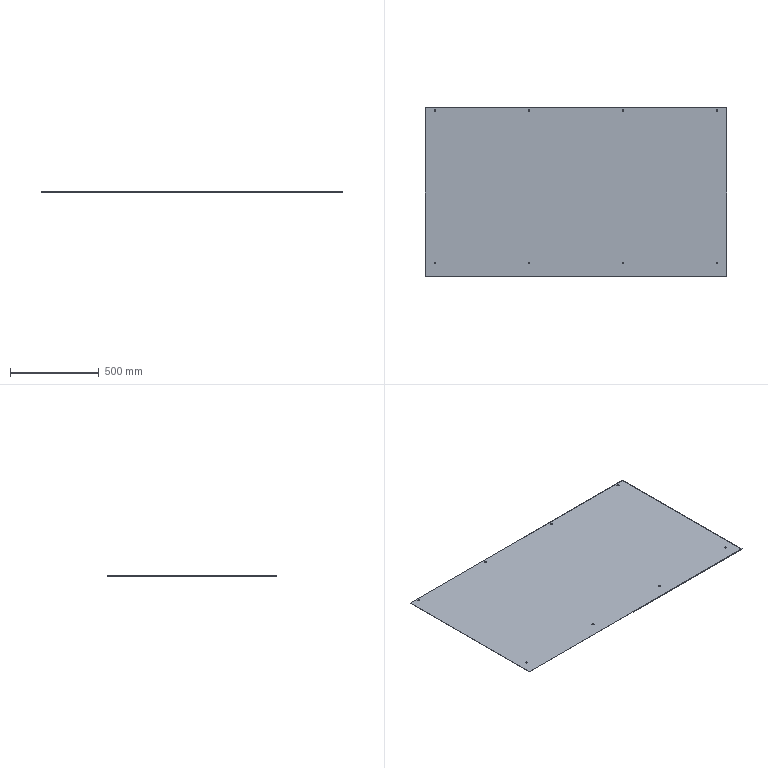Part | SolidWorks | features ICE 2, Extrusion 1 | 1 solid | 24 faces | box 1700 x 950 x 3 mm | volume 4835265 mm3 | cone 16 | plane 8
STEP:
#1=CARTESIAN_POINT('',(-261.75,460.,3.));
#2=VERTEX_POINT('',#1);
#3=CARTESIAN_POINT('',(-268.25,460.,3.));
#4=VERTEX_POINT('',#3);
#5=CARTESIAN_POINT('',(-265.,460.,3.));
#6=DIRECTION('',(0.,0.,1.));
#7=DIRECTION('',(1.,0.,0.));
#8=AXIS2_PLACEMENT_3D('',#5,#6,#7);
#9=CIRCLE('',#8,3.25);
#10=EDGE_CURVE('',#2,#4,#9,.T.);
#11=ORIENTED_EDGE('',*,*,#10,.T.);
#12=CARTESIAN_POINT('',(-271.25,460.,0.));
#13=VERTEX_POINT('',#12);
#14=CARTESIAN_POINT('',(-268.25,460.,3.));
#15=DIRECTION('',(-0.7071,0.,-0.7071));
#16=VECTOR('',#15,1000.);
#17=LINE('',#14,#16);
#18=EDGE_CURVE('',#4,#13,#17,.T.);
#19=ORIENTED_EDGE('',*,*,#18,.T.);
#20=CARTESIAN_POINT('',(-258.75,460.,0.));
#21=VERTEX_POINT('',#20);
#22=CARTESIAN_POINT('',(-265.,460.,0.));
#23=DIRECTION('',(0.,0.,1.));
#24=DIRECTION('',(1.,0.,0.));
#25=AXIS2_PLACEMENT_3D('',#22,#23,#24);
#26=CIRCLE('',#25,6.25);
#27=EDGE_CURVE('',#21,#13,#26,.T.);
#28=ORIENTED_EDGE('',*,*,#27,.F.);
#29=CARTESIAN_POINT('',(-261.75,460.,3.));
#30=DIRECTION('',(0.7071,0.,-0.7071));
#31=VECTOR('',#30,1000.);
#32=LINE('',#29,#31);
#33=EDGE_CURVE('',#2,#21,#32,.T.);
#34=ORIENTED_EDGE('',*,*,#33,.F.);
#35=EDGE_LOOP('',(#11,#19,#28,#34));
#36=FACE_OUTER_BOUND('',#35,.T.);
#37=CARTESIAN_POINT('',(-265.,460.,3.));
#38=DIRECTION('',(0.,0.,-1.));
#39=DIRECTION('',(1.,0.,0.));
#40=AXIS2_PLACEMENT_3D('',#37,#38,#39);
#41=CONICAL_SURFACE('',#40,3.25,0.7854);
#42=ADVANCED_FACE('',(#36),#41,.F.);
#43=CARTESIAN_POINT('',(268.25,460.,3.));
#44=VERTEX_POINT('',#43);
#45=CARTESIAN_POINT('',(261.75,460.,3.));
#46=VERTEX_POINT('',#45);
#47=CARTESIAN_POINT('',(265.,460.,3.));
#48=DIRECTION('',(0.,0.,1.));
#49=DIRECTION('',(1.,0.,0.));
#50=AXIS2_PLACEMENT_3D('',#47,#48,#49);
#51=CIRCLE('',#50,3.25);
#52=EDGE_CURVE('',#44,#46,#51,.T.);
#53=ORIENTED_EDGE('',*,*,#52,.T.);
#54=CARTESIAN_POINT('',(258.75,460.,0.));
#55=VERTEX_POINT('',#54);
#56=CARTESIAN_POINT('',(261.75,460.,3.));
#57=DIRECTION('',(-0.7071,0.,-0.7071));
#58=VECTOR('',#57,1000.);
#59=LINE('',#56,#58);
#60=EDGE_CURVE('',#46,#55,#59,.T.);
#61=ORIENTED_EDGE('',*,*,#60,.T.);
#62=CARTESIAN_POINT('',(271.25,460.,0.));
#63=VERTEX_POINT('',#62);
#64=CARTESIAN_POINT('',(265.,460.,0.));
#65=DIRECTION('',(0.,0.,1.));
#66=DIRECTION('',(1.,0.,0.));
#67=AXIS2_PLACEMENT_3D('',#64,#65,#66);
#68=CIRCLE('',#67,6.25);
#69=EDGE_CURVE('',#63,#55,#68,.T.);
#70=ORIENTED_EDGE('',*,*,#69,.F.);
#71=CARTESIAN_POINT('',(268.25,460.,3.));
#72=DIRECTION('',(0.7071,0.,-0.7071));
#73=VECTOR('',#72,1000.);
#74=LINE('',#71,#73);
#75=EDGE_CURVE('',#44,#63,#74,.T.);
#76=ORIENTED_EDGE('',*,*,#75,.F.);
#77=EDGE_LOOP('',(#53,#61,#70,#76));
#78=FACE_OUTER_BOUND('',#77,.T.);
#79=CARTESIAN_POINT('',(265.,460.,3.));
#80=DIRECTION('',(0.,0.,-1.));
#81=DIRECTION('',(1.,0.,0.));
#82=AXIS2_PLACEMENT_3D('',#79,#80,#81);
#83=CONICAL_SURFACE('',#82,3.25,0.7854);
#84=ADVANCED_FACE('',(#78),#83,.F.);
#85=CARTESIAN_POINT('',(798.25,460.,3.));
#86=VERTEX_POINT('',#85);
#87=CARTESIAN_POINT('',(791.75,460.,3.));
#88=VERTEX_POINT('',#87);
#89=CARTESIAN_POINT('',(795.,460.,3.));
#90=DIRECTION('',(0.,0.,1.));
#91=DIRECTION('',(1.,0.,0.));
#92=AXIS2_PLACEMENT_3D('',#89,#90,#91);
#93=CIRCLE('',#92,3.25);
#94=EDGE_CURVE('',#86,#88,#93,.T.);
#95=ORIENTED_EDGE('',*,*,#94,.T.);
#96=CARTESIAN_POINT('',(788.75,460.,0.));
#97=VERTEX_POINT('',#96);
#98=CARTESIAN_POINT('',(791.75,460.,3.));
#99=DIRECTION('',(-0.7071,0.,-0.7071));
#100=VECTOR('',#99,1000.);
#101=LINE('',#98,#100);
#102=EDGE_CURVE('',#88,#97,#101,.T.);
#103=ORIENTED_EDGE('',*,*,#102,.T.);
#104=CARTESIAN_POINT('',(801.25,460.,0.));
#105=VERTEX_POINT('',#104);
#106=CARTESIAN_POINT('',(795.,460.,0.));
#107=DIRECTION('',(0.,0.,1.));
#108=DIRECTION('',(1.,0.,0.));
#109=AXIS2_PLACEMENT_3D('',#106,#107,#108);
#110=CIRCLE('',#109,6.25);
#111=EDGE_CURVE('',#105,#97,#110,.T.);
#112=ORIENTED_EDGE('',*,*,#111,.F.);
#113=CARTESIAN_POINT('',(798.25,460.,3.));
#114=DIRECTION('',(0.7071,0.,-0.7071));
#115=VECTOR('',#114,1000.);
#116=LINE('',#113,#115);
#117=EDGE_CURVE('',#86,#105,#116,.T.);
#118=ORIENTED_EDGE('',*,*,#117,.F.);
#119=EDGE_LOOP('',(#95,#103,#112,#118));
#120=FACE_OUTER_BOUND('',#119,.T.);
#121=CARTESIAN_POINT('',(795.,460.,3.));
#122=DIRECTION('',(0.,0.,-1.));
#123=DIRECTION('',(1.,0.,0.));
#124=AXIS2_PLACEMENT_3D('',#121,#122,#123);
#125=CONICAL_SURFACE('',#124,3.25,0.7854);
#126=ADVANCED_FACE('',(#120),#125,.F.);
#127=CARTESIAN_POINT('',(798.25,-400.,3.));
#128=VERTEX_POINT('',#127);
#129=CARTESIAN_POINT('',(791.75,-400.,3.));
#130=VERTEX_POINT('',#129);
#131=CARTESIAN_POINT('',(795.,-400.,3.));
#132=DIRECTION('',(0.,0.,1.));
#133=DIRECTION('',(1.,0.,0.));
#134=AXIS2_PLACEMENT_3D('',#131,#132,#133);
#135=CIRCLE('',#134,3.25);
#136=EDGE_CURVE('',#128,#130,#135,.T.);
#137=ORIENTED_EDGE('',*,*,#136,.T.);
#138=CARTESIAN_POINT('',(788.75,-400.,0.));
#139=VERTEX_POINT('',#138);
#140=CARTESIAN_POINT('',(791.75,-400.,3.));
#141=DIRECTION('',(-0.7071,0.,-0.7071));
#142=VECTOR('',#141,1000.);
#143=LINE('',#140,#142);
#144=EDGE_CURVE('',#130,#139,#143,.T.);
#145=ORIENTED_EDGE('',*,*,#144,.T.);
#146=CARTESIAN_POINT('',(801.25,-400.,0.));
#147=VERTEX_POINT('',#146);
#148=CARTESIAN_POINT('',(795.,-400.,0.));
#149=DIRECTION('',(0.,0.,1.));
#150=DIRECTION('',(1.,0.,0.));
#151=AXIS2_PLACEMENT_3D('',#148,#149,#150);
#152=CIRCLE('',#151,6.25);
#153=EDGE_CURVE('',#147,#139,#152,.T.);
#154=ORIENTED_EDGE('',*,*,#153,.F.);
#155=CARTESIAN_POINT('',(798.25,-400.,3.));
#156=DIRECTION('',(0.7071,0.,-0.7071));
#157=VECTOR('',#156,1000.);
#158=LINE('',#155,#157);
#159=EDGE_CURVE('',#128,#147,#158,.T.);
#160=ORIENTED_EDGE('',*,*,#159,.F.);
#161=EDGE_LOOP('',(#137,#145,#154,#160));
#162=FACE_OUTER_BOUND('',#161,.T.);
#163=CARTESIAN_POINT('',(795.,-400.,3.));
#164=DIRECTION('',(0.,0.,-1.));
#165=DIRECTION('',(1.,0.,0.));
#166=AXIS2_PLACEMENT_3D('',#163,#164,#165);
#167=CONICAL_SURFACE('',#166,3.25,0.7854);
#168=ADVANCED_FACE('',(#162),#167,.F.);
#169=CARTESIAN_POINT('',(268.25,-400.,3.));
#170=VERTEX_POINT('',#169);
#171=CARTESIAN_POINT('',(261.75,-400.,3.));
#172=VERTEX_POINT('',#171);
#173=CARTESIAN_POINT('',(265.,-400.,3.));
#174=DIRECTION('',(0.,0.,1.));
#175=DIRECTION('',(1.,0.,0.));
#176=AXIS2_PLACEMENT_3D('',#173,#174,#175);
#177=CIRCLE('',#176,3.25);
#178=EDGE_CURVE('',#170,#172,#177,.T.);
#179=ORIENTED_EDGE('',*,*,#178,.T.);
#180=CARTESIAN_POINT('',(258.75,-400.,0.));
#181=VERTEX_POINT('',#180);
#182=CARTESIAN_POINT('',(261.75,-400.,3.));
#183=DIRECTION('',(-0.7071,0.,-0.7071));
#184=VECTOR('',#183,1000.);
#185=LINE('',#182,#184);
#186=EDGE_CURVE('',#172,#181,#185,.T.);
#187=ORIENTED_EDGE('',*,*,#186,.T.);
#188=CARTESIAN_POINT('',(271.25,-400.,0.));
#189=VERTEX_POINT('',#188);
#190=CARTESIAN_POINT('',(265.,-400.,0.));
#191=DIRECTION('',(0.,0.,1.));
#192=DIRECTION('',(1.,0.,0.));
#193=AXIS2_PLACEMENT_3D('',#190,#191,#192);
#194=CIRCLE('',#193,6.25);
#195=EDGE_CURVE('',#189,#181,#194,.T.);
#196=ORIENTED_EDGE('',*,*,#195,.F.);
#197=CARTESIAN_POINT('',(268.25,-400.,3.));
#198=DIRECTION('',(0.7071,0.,-0.7071));
#199=VECTOR('',#198,1000.);
#200=LINE('',#197,#199);
#201=EDGE_CURVE('',#170,#189,#200,.T.);
#202=ORIENTED_EDGE('',*,*,#201,.F.);
#203=EDGE_LOOP('',(#179,#187,#196,#202));
#204=FACE_OUTER_BOUND('',#203,.T.);
#205=CARTESIAN_POINT('',(265.,-400.,3.));
#206=DIRECTION('',(0.,0.,-1.));
#207=DIRECTION('',(1.,0.,0.));
#208=AXIS2_PLACEMENT_3D('',#205,#206,#207);
#209=CONICAL_SURFACE('',#208,3.25,0.7854);
#210=ADVANCED_FACE('',(#204),#209,.F.);
#211=CARTESIAN_POINT('',(-261.75,-400.,3.));
#212=VERTEX_POINT('',#211);
#213=CARTESIAN_POINT('',(-268.25,-400.,3.));
#214=VERTEX_POINT('',#213);
#215=CARTESIAN_POINT('',(-265.,-400.,3.));
#216=DIRECTION('',(0.,0.,1.));
#217=DIRECTION('',(1.,0.,0.));
#218=AXIS2_PLACEMENT_3D('',#215,#216,#217);
#219=CIRCLE('',#218,3.25);
#220=EDGE_CURVE('',#212,#214,#219,.T.);
#221=ORIENTED_EDGE('',*,*,#220,.T.);
#222=CARTESIAN_POINT('',(-271.25,-400.,0.));
#223=VERTEX_POINT('',#222);
#224=CARTESIAN_POINT('',(-268.25,-400.,3.));
#225=DIRECTION('',(-0.7071,0.,-0.7071));
#226=VECTOR('',#225,1000.);
#227=LINE('',#224,#226);
#228=EDGE_CURVE('',#214,#223,#227,.T.);
#229=ORIENTED_EDGE('',*,*,#228,.T.);
#230=CARTESIAN_POINT('',(-258.75,-400.,0.));
#231=VERTEX_POINT('',#230);
#232=CARTESIAN_POINT('',(-265.,-400.,0.));
#233=DIRECTION('',(0.,0.,1.));
#234=DIRECTION('',(1.,0.,0.));
#235=AXIS2_PLACEMENT_3D('',#232,#233,#234);
#236=CIRCLE('',#235,6.25);
#237=EDGE_CURVE('',#231,#223,#236,.T.);
#238=ORIENTED_EDGE('',*,*,#237,.F.);
#239=CARTESIAN_POINT('',(-261.75,-400.,3.));
#240=DIRECTION('',(0.7071,0.,-0.7071));
#241=VECTOR('',#240,1000.);
#242=LINE('',#239,#241);
#243=EDGE_CURVE('',#212,#231,#242,.T.);
#244=ORIENTED_EDGE('',*,*,#243,.F.);
#245=EDGE_LOOP('',(#221,#229,#238,#244));
#246=FACE_OUTER_BOUND('',#245,.T.);
#247=CARTESIAN_POINT('',(-265.,-400.,3.));
#248=DIRECTION('',(0.,0.,-1.));
#249=DIRECTION('',(1.,0.,0.));
#250=AXIS2_PLACEMENT_3D('',#247,#248,#249);
#251=CONICAL_SURFACE('',#250,3.25,0.7854);
#252=ADVANCED_FACE('',(#246),#251,.F.);
#253=CARTESIAN_POINT('',(-791.75,-400.,3.));
#254=VERTEX_POINT('',#253);
#255=CARTESIAN_POINT('',(-798.25,-400.,3.));
#256=VERTEX_POINT('',#255);
#257=CARTESIAN_POINT('',(-795.,-400.,3.));
#258=DIRECTION('',(0.,0.,1.));
#259=DIRECTION('',(1.,0.,0.));
#260=AXIS2_PLACEMENT_3D('',#257,#258,#259);
#261=CIRCLE('',#260,3.25);
#262=EDGE_CURVE('',#254,#256,#261,.T.);
#263=ORIENTED_EDGE('',*,*,#262,.T.);
#264=CARTESIAN_POINT('',(-801.25,-400.,0.));
#265=VERTEX_POINT('',#264);
#266=CARTESIAN_POINT('',(-798.25,-400.,3.));
#267=DIRECTION('',(-0.7071,0.,-0.7071));
#268=VECTOR('',#267,1000.);
#269=LINE('',#266,#268);
#270=EDGE_CURVE('',#256,#265,#269,.T.);
#271=ORIENTED_EDGE('',*,*,#270,.T.);
#272=CARTESIAN_POINT('',(-788.75,-400.,0.));
#273=VERTEX_POINT('',#272);
#274=CARTESIAN_POINT('',(-795.,-400.,0.));
#275=DIRECTION('',(0.,0.,1.));
#276=DIRECTION('',(1.,0.,0.));
#277=AXIS2_PLACEMENT_3D('',#274,#275,#276);
#278=CIRCLE('',#277,6.25);
#279=EDGE_CURVE('',#273,#265,#278,.T.);
#280=ORIENTED_EDGE('',*,*,#279,.F.);
#281=CARTESIAN_POINT('',(-791.75,-400.,3.));
#282=DIRECTION('',(0.7071,0.,-0.7071));
#283=VECTOR('',#282,1000.);
#284=LINE('',#281,#283);
#285=EDGE_CURVE('',#254,#273,#284,.T.);
#286=ORIENTED_EDGE('',*,*,#285,.F.);
#287=EDGE_LOOP('',(#263,#271,#280,#286));
#288=FACE_OUTER_BOUND('',#287,.T.);
#289=CARTESIAN_POINT('',(-795.,-400.,3.));
#290=DIRECTION('',(0.,0.,-1.));
#291=DIRECTION('',(1.,0.,0.));
#292=AXIS2_PLACEMENT_3D('',#289,#290,#291);
#293=CONICAL_SURFACE('',#292,3.25,0.7854);
#294=ADVANCED_FACE('',(#288),#293,.F.);
#295=CARTESIAN_POINT('',(-791.75,460.,3.));
#296=VERTEX_POINT('',#295);
#297=CARTESIAN_POINT('',(-798.25,460.,3.));
#298=VERTEX_POINT('',#297);
#299=CARTESIAN_POINT('',(-795.,460.,3.));
#300=DIRECTION('',(0.,0.,1.));
#301=DIRECTION('',(1.,0.,0.));
#302=AXIS2_PLACEMENT_3D('',#299,#300,#301);
#303=CIRCLE('',#302,3.25);
#304=EDGE_CURVE('',#296,#298,#303,.T.);
#305=ORIENTED_EDGE('',*,*,#304,.T.);
#306=CARTESIAN_POINT('',(-801.25,460.,0.));
#307=VERTEX_POINT('',#306);
#308=CARTESIAN_POINT('',(-798.25,460.,3.));
#309=DIRECTION('',(-0.7071,0.,-0.7071));
#310=VECTOR('',#309,1000.);
#311=LINE('',#308,#310);
#312=EDGE_CURVE('',#298,#307,#311,.T.);
#313=ORIENTED_EDGE('',*,*,#312,.T.);
#314=CARTESIAN_POINT('',(-788.75,460.,0.));
#315=VERTEX_POINT('',#314);
#316=CARTESIAN_POINT('',(-795.,460.,0.));
#317=DIRECTION('',(0.,0.,1.));
#318=DIRECTION('',(1.,0.,0.));
#319=AXIS2_PLACEMENT_3D('',#316,#317,#318);
#320=CIRCLE('',#319,6.25);
#321=EDGE_CURVE('',#315,#307,#320,.T.);
#322=ORIENTED_EDGE('',*,*,#321,.F.);
#323=CARTESIAN_POINT('',(-791.75,460.,3.));
#324=DIRECTION('',(0.7071,0.,-0.7071));
#325=VECTOR('',#324,1000.);
#326=LINE('',#323,#325);
#327=EDGE_CURVE('',#296,#315,#326,.T.);
#328=ORIENTED_EDGE('',*,*,#327,.F.);
#329=EDGE_LOOP('',(#305,#313,#322,#328));
#330=FACE_OUTER_BOUND('',#329,.T.);
#331=CARTESIAN_POINT('',(-795.,460.,3.));
#332=DIRECTION('',(0.,0.,-1.));
#333=DIRECTION('',(1.,0.,0.));
#334=AXIS2_PLACEMENT_3D('',#331,#332,#333);
#335=CONICAL_SURFACE('',#334,3.25,0.7854);
#336=ADVANCED_FACE('',(#330),#335,.F.);
#337=CARTESIAN_POINT('',(850.,475.,1.5));
#338=VERTEX_POINT('',#337);
#339=CARTESIAN_POINT('',(850.,-475.,1.5));
#340=VERTEX_POINT('',#339);
#341=CARTESIAN_POINT('',(850.,475.,1.5));
#342=DIRECTION('',(0.,-1.,0.));
#343=VECTOR('',#342,1000.);
#344=LINE('',#341,#343);
#345=EDGE_CURVE('',#338,#340,#344,.T.);
#346=ORIENTED_EDGE('',*,*,#345,.F.);
#347=CARTESIAN_POINT('',(850.,475.,3.));
#348=VERTEX_POINT('',#347);
#349=CARTESIAN_POINT('',(850.,475.,3.));
#350=DIRECTION('',(0.,0.,-1.));
#351=VECTOR('',#350,1000.);
#352=LINE('',#349,#351);
#353=EDGE_CURVE('',#348,#338,#352,.T.);
#354=ORIENTED_EDGE('',*,*,#353,.F.);
#355=CARTESIAN_POINT('',(850.,-475.,3.));
#356=VERTEX_POINT('',#355);
#357=CARTESIAN_POINT('',(850.,475.,3.));
#358=DIRECTION('',(0.,1.,0.));
#359=VECTOR('',#358,1000.);
#360=LINE('',#357,#359);
#361=EDGE_CURVE('',#356,#348,#360,.T.);
#362=ORIENTED_EDGE('',*,*,#361,.F.);
#363=CARTESIAN_POINT('',(850.,-475.,3.));
#364=DIRECTION('',(0.,0.,-1.));
#365=VECTOR('',#364,1000.);
#366=LINE('',#363,#365);
#367=EDGE_CURVE('',#356,#340,#366,.T.);
#368=ORIENTED_EDGE('',*,*,#367,.T.);
#369=EDGE_LOOP('',(#346,#354,#362,#368));
#370=FACE_OUTER_BOUND('',#369,.T.);
#371=CARTESIAN_POINT('',(850.,475.,3.));
#372=DIRECTION('',(-1.,0.,0.));
#373=DIRECTION('',(0.,-1.,0.));
#374=AXIS2_PLACEMENT_3D('',#371,#372,#373);
#375=PLANE('',#374);
#376=ADVANCED_FACE('',(#370),#375,.F.);
#377=CARTESIAN_POINT('',(844.402,475.,0.));
#378=VERTEX_POINT('',#377);
#379=CARTESIAN_POINT('',(-844.402,475.,0.));
#380=VERTEX_POINT('',#379);
#381=CARTESIAN_POINT('',(-850.,475.,0.));
#382=DIRECTION('',(-1.,0.,0.));
#383=VECTOR('',#382,1000.);
#384=LINE('',#381,#383);
#385=EDGE_CURVE('',#378,#380,#384,.T.);
#386=ORIENTED_EDGE('',*,*,#385,.T.);
#387=CARTESIAN_POINT('',(-850.,475.,1.5));
#388=VERTEX_POINT('',#387);
#389=CARTESIAN_POINT('',(-844.402,475.,0.));
#390=DIRECTION('',(-0.9659,0.,0.2588));
#391=VECTOR('',#390,1000.);
#392=LINE('',#389,#391);
#393=EDGE_CURVE('',#380,#388,#392,.T.);
#394=ORIENTED_EDGE('',*,*,#393,.T.);
#395=CARTESIAN_POINT('',(-850.,475.,3.));
#396=VERTEX_POINT('',#395);
#397=CARTESIAN_POINT('',(-850.,475.,3.));
#398=DIRECTION('',(0.,0.,-1.));
#399=VECTOR('',#398,1000.);
#400=LINE('',#397,#399);
#401=EDGE_CURVE('',#396,#388,#400,.T.);
#402=ORIENTED_EDGE('',*,*,#401,.F.);
#403=CARTESIAN_POINT('',(-850.,475.,3.));
#404=DIRECTION('',(-1.,0.,0.));
#405=VECTOR('',#404,1000.);
#406=LINE('',#403,#405);
#407=EDGE_CURVE('',#348,#396,#406,.T.);
#408=ORIENTED_EDGE('',*,*,#407,.F.);
#409=ORIENTED_EDGE('',*,*,#353,.T.);
#410=CARTESIAN_POINT('',(844.402,475.,0.));
#411=DIRECTION('',(0.9659,0.,0.2588));
#412=VECTOR('',#411,1000.);
#413=LINE('',#410,#412);
#414=EDGE_CURVE('',#378,#338,#413,.T.);
#415=ORIENTED_EDGE('',*,*,#414,.F.);
#416=EDGE_LOOP('',(#386,#394,#402,#408,#409,#415));
#417=FACE_OUTER_BOUND('',#416,.T.);
#418=CARTESIAN_POINT('',(-850.,475.,3.));
#419=DIRECTION('',(0.,-1.,0.));
#420=DIRECTION('',(0.,0.,-1.));
#421=AXIS2_PLACEMENT_3D('',#418,#419,#420);
#422=PLANE('',#421);
#423=ADVANCED_FACE('',(#417),#422,.F.);
#424=CARTESIAN_POINT('',(-850.,-475.,3.));
#425=VERTEX_POINT('',#424);
#426=CARTESIAN_POINT('',(-850.,-475.,1.5));
#427=VERTEX_POINT('',#426);
#428=CARTESIAN_POINT('',(-850.,-475.,3.));
#429=DIRECTION('',(0.,0.,-1.));
#430=VECTOR('',#429,1000.);
#431=LINE('',#428,#430);
#432=EDGE_CURVE('',#425,#427,#431,.T.);
#433=ORIENTED_EDGE('',*,*,#432,.T.);
#434=CARTESIAN_POINT('',(-844.402,-475.,0.));
#435=VERTEX_POINT('',#434);
#436=CARTESIAN_POINT('',(-844.402,-475.,0.));
#437=DIRECTION('',(-0.9659,0.,0.2588));
#438=VECTOR('',#437,1000.);
#439=LINE('',#436,#438);
#440=EDGE_CURVE('',#435,#427,#439,.T.);
#441=ORIENTED_EDGE('',*,*,#440,.F.);
#442=CARTESIAN_POINT('',(844.402,-475.,0.));
#443=VERTEX_POINT('',#442);
#444=CARTESIAN_POINT('',(-850.,-475.,0.));
#445=DIRECTION('',(1.,0.,0.));
#446=VECTOR('',#445,1000.);
#447=LINE('',#444,#446);
#448=EDGE_CURVE('',#435,#443,#447,.T.);
#449=ORIENTED_EDGE('',*,*,#448,.T.);
#450=CARTESIAN_POINT('',(844.402,-475.,0.));
#451=DIRECTION('',(0.9659,0.,0.2588));
#452=VECTOR('',#451,1000.);
#453=LINE('',#450,#452);
#454=EDGE_CURVE('',#443,#340,#453,.T.);
#455=ORIENTED_EDGE('',*,*,#454,.T.);
#456=ORIENTED_EDGE('',*,*,#367,.F.);
#457=CARTESIAN_POINT('',(-850.,-475.,3.));
#458=DIRECTION('',(1.,0.,0.));
#459=VECTOR('',#458,1000.);
#460=LINE('',#457,#459);
#461=EDGE_CURVE('',#425,#356,#460,.T.);
#462=ORIENTED_EDGE('',*,*,#461,.F.);
#463=EDGE_LOOP('',(#433,#441,#449,#455,#456,#462));
#464=FACE_OUTER_BOUND('',#463,.T.);
#465=CARTESIAN_POINT('',(-850.,-475.,3.));
#466=DIRECTION('',(0.,1.,0.));
#467=DIRECTION('',(0.,0.,1.));
#468=AXIS2_PLACEMENT_3D('',#465,#466,#467);
#469=PLANE('',#468);
#470=ADVANCED_FACE('',(#464),#469,.F.);
#471=ORIENTED_EDGE('',*,*,#321,.T.);
#472=CARTESIAN_POINT('',(-795.,460.,0.));
#473=DIRECTION('',(0.,0.,1.));
#474=DIRECTION('',(1.,0.,0.));
#475=AXIS2_PLACEMENT_3D('',#472,#473,#474);
#476=CIRCLE('',#475,6.25);
#477=EDGE_CURVE('',#307,#315,#476,.T.);
#478=ORIENTED_EDGE('',*,*,#477,.T.);
#479=EDGE_LOOP('',(#471,#478));
#480=FACE_BOUND('',#479,.T.);
#481=ORIENTED_EDGE('',*,*,#279,.T.);
#482=CARTESIAN_POINT('',(-795.,-400.,0.));
#483=DIRECTION('',(0.,0.,1.));
#484=DIRECTION('',(1.,0.,0.));
#485=AXIS2_PLACEMENT_3D('',#482,#483,#484);
#486=CIRCLE('',#485,6.25);
#487=EDGE_CURVE('',#265,#273,#486,.T.);
#488=ORIENTED_EDGE('',*,*,#487,.T.);
#489=EDGE_LOOP('',(#481,#488));
#490=FACE_BOUND('',#489,.T.);
#491=ORIENTED_EDGE('',*,*,#237,.T.);
#492=CARTESIAN_POINT('',(-265.,-400.,0.));
#493=DIRECTION('',(0.,0.,1.));
#494=DIRECTION('',(1.,0.,0.));
#495=AXIS2_PLACEMENT_3D('',#492,#493,#494);
#496=CIRCLE('',#495,6.25);
#497=EDGE_CURVE('',#223,#231,#496,.T.);
#498=ORIENTED_EDGE('',*,*,#497,.T.);
#499=EDGE_LOOP('',(#491,#498));
#500=FACE_BOUND('',#499,.T.);
#501=ORIENTED_EDGE('',*,*,#195,.T.);
#502=CARTESIAN_POINT('',(265.,-400.,0.));
#503=DIRECTION('',(0.,0.,1.));
#504=DIRECTION('',(1.,0.,0.));
#505=AXIS2_PLACEMENT_3D('',#502,#503,#504);
#506=CIRCLE('',#505,6.25);
#507=EDGE_CURVE('',#181,#189,#506,.T.);
#508=ORIENTED_EDGE('',*,*,#507,.T.);
#509=EDGE_LOOP('',(#501,#508));
#510=FACE_BOUND('',#509,.T.);
#511=ORIENTED_EDGE('',*,*,#153,.T.);
#512=CARTESIAN_POINT('',(795.,-400.,0.));
#513=DIRECTION('',(0.,0.,1.));
#514=DIRECTION('',(1.,0.,0.));
#515=AXIS2_PLACEMENT_3D('',#512,#513,#514);
#516=CIRCLE('',#515,6.25);
#517=EDGE_CURVE('',#139,#147,#516,.T.);
#518=ORIENTED_EDGE('',*,*,#517,.T.);
#519=EDGE_LOOP('',(#511,#518));
#520=FACE_BOUND('',#519,.T.);
#521=ORIENTED_EDGE('',*,*,#111,.T.);
#522=CARTESIAN_POINT('',(795.,460.,0.));
#523=DIRECTION('',(0.,0.,1.));
#524=DIRECTION('',(1.,0.,0.));
#525=AXIS2_PLACEMENT_3D('',#522,#523,#524);
#526=CIRCLE('',#525,6.25);
#527=EDGE_CURVE('',#97,#105,#526,.T.);
#528=ORIENTED_EDGE('',*,*,#527,.T.);
#529=EDGE_LOOP('',(#521,#528));
#530=FACE_BOUND('',#529,.T.);
#531=ORIENTED_EDGE('',*,*,#69,.T.);
#532=CARTESIAN_POINT('',(265.,460.,0.));
#533=DIRECTION('',(0.,0.,1.));
#534=DIRECTION('',(1.,0.,0.));
#535=AXIS2_PLACEMENT_3D('',#532,#533,#534);
#536=CIRCLE('',#535,6.25);
#537=EDGE_CURVE('',#55,#63,#536,.T.);
#538=ORIENTED_EDGE('',*,*,#537,.T.);
#539=EDGE_LOOP('',(#531,#538));
#540=FACE_BOUND('',#539,.T.);
#541=ORIENTED_EDGE('',*,*,#27,.T.);
#542=CARTESIAN_POINT('',(-265.,460.,0.));
#543=DIRECTION('',(0.,0.,1.));
#544=DIRECTION('',(1.,0.,0.));
#545=AXIS2_PLACEMENT_3D('',#542,#543,#544);
#546=CIRCLE('',#545,6.25);
#547=EDGE_CURVE('',#13,#21,#546,.T.);
#548=ORIENTED_EDGE('',*,*,#547,.T.);
#549=EDGE_LOOP('',(#541,#548));
#550=FACE_BOUND('',#549,.T.);
#551=ORIENTED_EDGE('',*,*,#448,.F.);
#552=CARTESIAN_POINT('',(-844.402,475.,0.));
#553=DIRECTION('',(0.,-1.,0.));
#554=VECTOR('',#553,1000.);
#555=LINE('',#552,#554);
#556=EDGE_CURVE('',#380,#435,#555,.T.);
#557=ORIENTED_EDGE('',*,*,#556,.F.);
#558=ORIENTED_EDGE('',*,*,#385,.F.);
#559=CARTESIAN_POINT('',(844.402,475.,0.));
#560=DIRECTION('',(0.,-1.,0.));
#561=VECTOR('',#560,1000.);
#562=LINE('',#559,#561);
#563=EDGE_CURVE('',#378,#443,#562,.T.);
#564=ORIENTED_EDGE('',*,*,#563,.T.);
#565=EDGE_LOOP('',(#551,#557,#558,#564));
#566=FACE_OUTER_BOUND('',#565,.T.);
#567=CARTESIAN_POINT('',(0.,0.,0.));
#568=DIRECTION('',(0.,0.,1.));
#569=DIRECTION('',(1.,0.,0.));
#570=AXIS2_PLACEMENT_3D('',#567,#568,#569);
#571=PLANE('',#570);
#572=ADVANCED_FACE('',(#480,#490,#500,#510,#520,#530,#540,#550,#566),#571,.F.);
#573=ORIENTED_EDGE('',*,*,#401,.T.);
#574=CARTESIAN_POINT('',(-850.,475.,1.5));
#575=DIRECTION('',(0.,-1.,0.));
#576=VECTOR('',#575,1000.);
#577=LINE('',#574,#576);
#578=EDGE_CURVE('',#388,#427,#577,.T.);
#579=ORIENTED_EDGE('',*,*,#578,.T.);
#580=ORIENTED_EDGE('',*,*,#432,.F.);
#581=CARTESIAN_POINT('',(-850.,475.,3.));
#582=DIRECTION('',(0.,-1.,0.));
#583=VECTOR('',#582,1000.);
#584=LINE('',#581,#583);
#585=EDGE_CURVE('',#396,#425,#584,.T.);
#586=ORIENTED_EDGE('',*,*,#585,.F.);
#587=EDGE_LOOP('',(#573,#579,#580,#586));
#588=FACE_OUTER_BOUND('',#587,.T.);
#589=CARTESIAN_POINT('',(-850.,475.,3.));
#590=DIRECTION('',(1.,0.,0.));
#591=DIRECTION('',(0.,0.,-1.));
#592=AXIS2_PLACEMENT_3D('',#589,#590,#591);
#593=PLANE('',#592);
#594=ADVANCED_FACE('',(#588),#593,.F.);
#595=ORIENTED_EDGE('',*,*,#10,.F.);
#596=CARTESIAN_POINT('',(-265.,460.,3.));
#597=DIRECTION('',(0.,0.,1.));
#598=DIRECTION('',(1.,0.,0.));
#599=AXIS2_PLACEMENT_3D('',#596,#597,#598);
#600=CIRCLE('',#599,3.25);
#601=EDGE_CURVE('',#4,#2,#600,.T.);
#602=ORIENTED_EDGE('',*,*,#601,.F.);
#603=EDGE_LOOP('',(#595,#602));
#604=FACE_BOUND('',#603,.T.);
#605=ORIENTED_EDGE('',*,*,#52,.F.);
#606=CARTESIAN_POINT('',(265.,460.,3.));
#607=DIRECTION('',(0.,0.,1.));
#608=DIRECTION('',(1.,0.,0.));
#609=AXIS2_PLACEMENT_3D('',#606,#607,#608);
#610=CIRCLE('',#609,3.25);
#611=EDGE_CURVE('',#46,#44,#610,.T.);
#612=ORIENTED_EDGE('',*,*,#611,.F.);
#613=EDGE_LOOP('',(#605,#612));
#614=FACE_BOUND('',#613,.T.);
#615=ORIENTED_EDGE('',*,*,#94,.F.);
#616=CARTESIAN_POINT('',(795.,460.,3.));
#617=DIRECTION('',(0.,0.,1.));
#618=DIRECTION('',(1.,0.,0.));
#619=AXIS2_PLACEMENT_3D('',#616,#617,#618);
#620=CIRCLE('',#619,3.25);
#621=EDGE_CURVE('',#88,#86,#620,.T.);
#622=ORIENTED_EDGE('',*,*,#621,.F.);
#623=EDGE_LOOP('',(#615,#622));
#624=FACE_BOUND('',#623,.T.);
#625=ORIENTED_EDGE('',*,*,#136,.F.);
#626=CARTESIAN_POINT('',(795.,-400.,3.));
#627=DIRECTION('',(0.,0.,1.));
#628=DIRECTION('',(1.,0.,0.));
#629=AXIS2_PLACEMENT_3D('',#626,#627,#628);
#630=CIRCLE('',#629,3.25);
#631=EDGE_CURVE('',#130,#128,#630,.T.);
#632=ORIENTED_EDGE('',*,*,#631,.F.);
#633=EDGE_LOOP('',(#625,#632));
#634=FACE_BOUND('',#633,.T.);
#635=ORIENTED_EDGE('',*,*,#178,.F.);
#636=CARTESIAN_POINT('',(265.,-400.,3.));
#637=DIRECTION('',(0.,0.,1.));
#638=DIRECTION('',(1.,0.,0.));
#639=AXIS2_PLACEMENT_3D('',#636,#637,#638);
#640=CIRCLE('',#639,3.25);
#641=EDGE_CURVE('',#172,#170,#640,.T.);
#642=ORIENTED_EDGE('',*,*,#641,.F.);
#643=EDGE_LOOP('',(#635,#642));
#644=FACE_BOUND('',#643,.T.);
#645=ORIENTED_EDGE('',*,*,#220,.F.);
#646=CARTESIAN_POINT('',(-265.,-400.,3.));
#647=DIRECTION('',(0.,0.,1.));
#648=DIRECTION('',(1.,0.,0.));
#649=AXIS2_PLACEMENT_3D('',#646,#647,#648);
#650=CIRCLE('',#649,3.25);
#651=EDGE_CURVE('',#214,#212,#650,.T.);
#652=ORIENTED_EDGE('',*,*,#651,.F.);
#653=EDGE_LOOP('',(#645,#652));
#654=FACE_BOUND('',#653,.T.);
#655=ORIENTED_EDGE('',*,*,#262,.F.);
#656=CARTESIAN_POINT('',(-795.,-400.,3.));
#657=DIRECTION('',(0.,0.,1.));
#658=DIRECTION('',(1.,0.,0.));
#659=AXIS2_PLACEMENT_3D('',#656,#657,#658);
#660=CIRCLE('',#659,3.25);
#661=EDGE_CURVE('',#256,#254,#660,.T.);
#662=ORIENTED_EDGE('',*,*,#661,.F.);
#663=EDGE_LOOP('',(#655,#662));
#664=FACE_BOUND('',#663,.T.);
#665=ORIENTED_EDGE('',*,*,#304,.F.);
#666=CARTESIAN_POINT('',(-795.,460.,3.));
#667=DIRECTION('',(0.,0.,1.));
#668=DIRECTION('',(1.,0.,0.));
#669=AXIS2_PLACEMENT_3D('',#666,#667,#668);
#670=CIRCLE('',#669,3.25);
#671=EDGE_CURVE('',#298,#296,#670,.T.);
#672=ORIENTED_EDGE('',*,*,#671,.F.);
#673=EDGE_LOOP('',(#665,#672));
#674=FACE_BOUND('',#673,.T.);
#675=ORIENTED_EDGE('',*,*,#361,.T.);
#676=ORIENTED_EDGE('',*,*,#407,.T.);
#677=ORIENTED_EDGE('',*,*,#585,.T.);
#678=ORIENTED_EDGE('',*,*,#461,.T.);
#679=EDGE_LOOP('',(#675,#676,#677,#678));
#680=FACE_OUTER_BOUND('',#679,.T.);
#681=CARTESIAN_POINT('',(0.,0.,3.));
#682=DIRECTION('',(0.,0.,1.));
#683=DIRECTION('',(1.,0.,0.));
#684=AXIS2_PLACEMENT_3D('',#681,#682,#683);
#685=PLANE('',#684);
#686=ADVANCED_FACE('',(#604,#614,#624,#634,#644,#654,#664,#674,#680),#685,.T.);
#687=ORIENTED_EDGE('',*,*,#312,.F.);
#688=ORIENTED_EDGE('',*,*,#671,.T.);
#689=ORIENTED_EDGE('',*,*,#327,.T.);
#690=ORIENTED_EDGE('',*,*,#477,.F.);
#691=EDGE_LOOP('',(#687,#688,#689,#690));
#692=FACE_OUTER_BOUND('',#691,.T.);
#693=CARTESIAN_POINT('',(-795.,460.,3.));
#694=DIRECTION('',(0.,0.,-1.));
#695=DIRECTION('',(1.,0.,0.));
#696=AXIS2_PLACEMENT_3D('',#693,#694,#695);
#697=CONICAL_SURFACE('',#696,3.25,0.7854);
#698=ADVANCED_FACE('',(#692),#697,.F.);
#699=ORIENTED_EDGE('',*,*,#270,.F.);
#700=ORIENTED_EDGE('',*,*,#661,.T.);
#701=ORIENTED_EDGE('',*,*,#285,.T.);
#702=ORIENTED_EDGE('',*,*,#487,.F.);
#703=EDGE_LOOP('',(#699,#700,#701,#702));
#704=FACE_OUTER_BOUND('',#703,.T.);
#705=CARTESIAN_POINT('',(-795.,-400.,3.));
#706=DIRECTION('',(0.,0.,-1.));
#707=DIRECTION('',(1.,0.,0.));
#708=AXIS2_PLACEMENT_3D('',#705,#706,#707);
#709=CONICAL_SURFACE('',#708,3.25,0.7854);
#710=ADVANCED_FACE('',(#704),#709,.F.);
#711=ORIENTED_EDGE('',*,*,#228,.F.);
#712=ORIENTED_EDGE('',*,*,#651,.T.);
#713=ORIENTED_EDGE('',*,*,#243,.T.);
#714=ORIENTED_EDGE('',*,*,#497,.F.);
#715=EDGE_LOOP('',(#711,#712,#713,#714));
#716=FACE_OUTER_BOUND('',#715,.T.);
#717=CARTESIAN_POINT('',(-265.,-400.,3.));
#718=DIRECTION('',(0.,0.,-1.));
#719=DIRECTION('',(1.,0.,0.));
#720=AXIS2_PLACEMENT_3D('',#717,#718,#719);
#721=CONICAL_SURFACE('',#720,3.25,0.7854);
#722=ADVANCED_FACE('',(#716),#721,.F.);
#723=ORIENTED_EDGE('',*,*,#186,.F.);
#724=ORIENTED_EDGE('',*,*,#641,.T.);
#725=ORIENTED_EDGE('',*,*,#201,.T.);
#726=ORIENTED_EDGE('',*,*,#507,.F.);
#727=EDGE_LOOP('',(#723,#724,#725,#726));
#728=FACE_OUTER_BOUND('',#727,.T.);
#729=CARTESIAN_POINT('',(265.,-400.,3.));
#730=DIRECTION('',(0.,0.,-1.));
#731=DIRECTION('',(1.,0.,0.));
#732=AXIS2_PLACEMENT_3D('',#729,#730,#731);
#733=CONICAL_SURFACE('',#732,3.25,0.7854);
#734=ADVANCED_FACE('',(#728),#733,.F.);
#735=ORIENTED_EDGE('',*,*,#144,.F.);
#736=ORIENTED_EDGE('',*,*,#631,.T.);
#737=ORIENTED_EDGE('',*,*,#159,.T.);
#738=ORIENTED_EDGE('',*,*,#517,.F.);
#739=EDGE_LOOP('',(#735,#736,#737,#738));
#740=FACE_OUTER_BOUND('',#739,.T.);
#741=CARTESIAN_POINT('',(795.,-400.,3.));
#742=DIRECTION('',(0.,0.,-1.));
#743=DIRECTION('',(1.,0.,0.));
#744=AXIS2_PLACEMENT_3D('',#741,#742,#743);
#745=CONICAL_SURFACE('',#744,3.25,0.7854);
#746=ADVANCED_FACE('',(#740),#745,.F.);
#747=ORIENTED_EDGE('',*,*,#102,.F.);
#748=ORIENTED_EDGE('',*,*,#621,.T.);
#749=ORIENTED_EDGE('',*,*,#117,.T.);
#750=ORIENTED_EDGE('',*,*,#527,.F.);
#751=EDGE_LOOP('',(#747,#748,#749,#750));
#752=FACE_OUTER_BOUND('',#751,.T.);
#753=CARTESIAN_POINT('',(795.,460.,3.));
#754=DIRECTION('',(0.,0.,-1.));
#755=DIRECTION('',(1.,0.,0.));
#756=AXIS2_PLACEMENT_3D('',#753,#754,#755);
#757=CONICAL_SURFACE('',#756,3.25,0.7854);
#758=ADVANCED_FACE('',(#752),#757,.F.);
#759=ORIENTED_EDGE('',*,*,#60,.F.);
#760=ORIENTED_EDGE('',*,*,#611,.T.);
#761=ORIENTED_EDGE('',*,*,#75,.T.);
#762=ORIENTED_EDGE('',*,*,#537,.F.);
#763=EDGE_LOOP('',(#759,#760,#761,#762));
#764=FACE_OUTER_BOUND('',#763,.T.);
#765=CARTESIAN_POINT('',(265.,460.,3.));
#766=DIRECTION('',(0.,0.,-1.));
#767=DIRECTION('',(1.,0.,0.));
#768=AXIS2_PLACEMENT_3D('',#765,#766,#767);
#769=CONICAL_SURFACE('',#768,3.25,0.7854);
#770=ADVANCED_FACE('',(#764),#769,.F.);
#771=ORIENTED_EDGE('',*,*,#18,.F.);
#772=ORIENTED_EDGE('',*,*,#601,.T.);
#773=ORIENTED_EDGE('',*,*,#33,.T.);
#774=ORIENTED_EDGE('',*,*,#547,.F.);
#775=EDGE_LOOP('',(#771,#772,#773,#774));
#776=FACE_OUTER_BOUND('',#775,.T.);
#777=CARTESIAN_POINT('',(-265.,460.,3.));
#778=DIRECTION('',(0.,0.,-1.));
#779=DIRECTION('',(1.,0.,0.));
#780=AXIS2_PLACEMENT_3D('',#777,#778,#779);
#781=CONICAL_SURFACE('',#780,3.25,0.7854);
#782=ADVANCED_FACE('',(#776),#781,.F.);
#783=ORIENTED_EDGE('',*,*,#454,.F.);
#784=ORIENTED_EDGE('',*,*,#563,.F.);
#785=ORIENTED_EDGE('',*,*,#414,.T.);
#786=ORIENTED_EDGE('',*,*,#345,.T.);
#787=EDGE_LOOP('',(#783,#784,#785,#786));
#788=FACE_OUTER_BOUND('',#787,.T.);
#789=CARTESIAN_POINT('',(844.402,475.,0.));
#790=DIRECTION('',(0.2588,0.,-0.9659));
#791=DIRECTION('',(-0.9659,0.,-0.2588));
#792=AXIS2_PLACEMENT_3D('',#789,#790,#791);
#793=PLANE('',#792);
#794=ADVANCED_FACE('',(#788),#793,.T.);
#795=ORIENTED_EDGE('',*,*,#440,.T.);
#796=ORIENTED_EDGE('',*,*,#578,.F.);
#797=ORIENTED_EDGE('',*,*,#393,.F.);
#798=ORIENTED_EDGE('',*,*,#556,.T.);
#799=EDGE_LOOP('',(#795,#796,#797,#798));
#800=FACE_OUTER_BOUND('',#799,.T.);
#801=CARTESIAN_POINT('',(-844.402,475.,0.));
#802=DIRECTION('',(0.2588,0.,0.9659));
#803=DIRECTION('',(0.9659,0.,-0.2588));
#804=AXIS2_PLACEMENT_3D('',#801,#802,#803);
#805=PLANE('',#804);
#806=ADVANCED_FACE('',(#800),#805,.F.);
#807=CLOSED_SHELL('',(#42,#84,#126,#168,#210,#252,#294,#336,#376,#423,#470,#572,#594,#686,#698,#710,#722,#734,#746,#758,#770,#782,#794,#806));
#808=MANIFOLD_SOLID_BREP('',#807);
#809=CARTESIAN_POINT('',(0.,0.,0.));
#810=DIRECTION('',(0.,0.,1.));
#811=DIRECTION('',(1.,0.,0.));
#812=AXIS2_PLACEMENT_3D('',#809,#810,#811);
#813=(LENGTH_UNIT()NAMED_UNIT(*)SI_UNIT(.MILLI.,.METRE.));
#814=UNCERTAINTY_MEASURE_WITH_UNIT(LENGTH_MEASURE(0.00001),#813,'','');
#815=(NAMED_UNIT(*)PLANE_ANGLE_UNIT()SI_UNIT($,.RADIAN.));
#816=(NAMED_UNIT(*)SI_UNIT($,.STERADIAN.)SOLID_ANGLE_UNIT());
#817=(GEOMETRIC_REPRESENTATION_CONTEXT(3)GLOBAL_UNCERTAINTY_ASSIGNED_CONTEXT((#814))GLOBAL_UNIT_ASSIGNED_CONTEXT((#813,#815,#816))REPRESENTATION_CONTEXT('',''));
#818=ADVANCED_BREP_SHAPE_REPRESENTATION('',(#808,#812),#817);